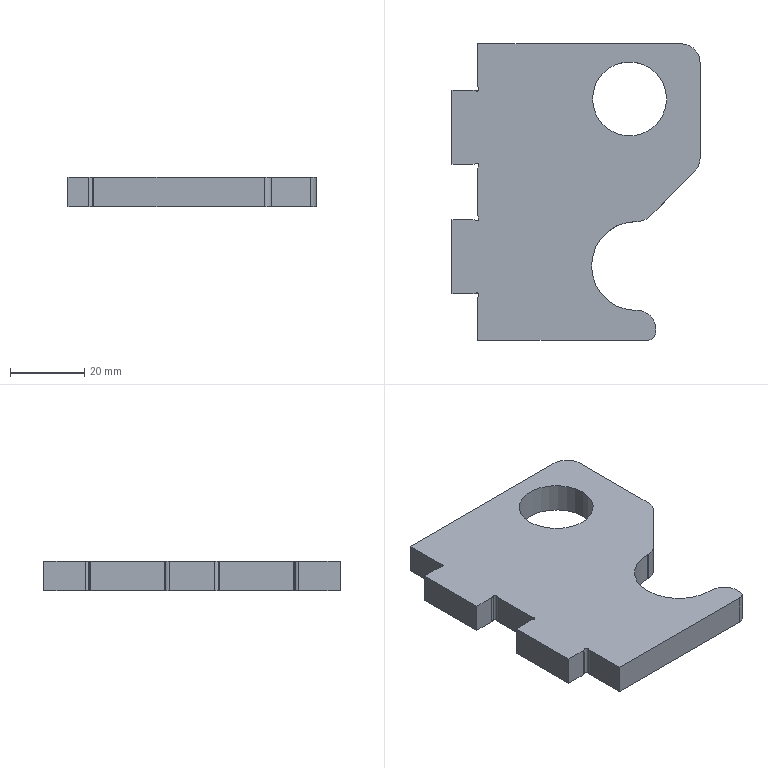Part | SolidWorks | features Fillet 2, Chamfer 1, FlatPattern 1, ICE 1, SMBaseFlange 1, SheetMetal 1 | 1 solid | 43 faces | box 67 x 80 x 8 mm | volume 31215 mm3 | cylinder 25 | plane 18 | commonest cylinder face diameters 4 x9 1 x8 10 x4 20 x2 24 x2
STEP:
#1=CARTESIAN_POINT('',(-1503.95,-7.25,0.));
#2=VERTEX_POINT('',#1);
#3=CARTESIAN_POINT('',(-1504.,-7.032,0.));
#4=VERTEX_POINT('',#3);
#5=CARTESIAN_POINT('',(-1504.45,-7.25,0.));
#6=DIRECTION('',(0.,0.,1.));
#7=DIRECTION('',(1.,0.,0.));
#8=AXIS2_PLACEMENT_3D('',#5,#6,#7);
#9=CIRCLE('',#8,0.5);
#10=EDGE_CURVE('',#2,#4,#9,.T.);
#11=ORIENTED_EDGE('',*,*,#10,.F.);
#12=CARTESIAN_POINT('',(-1503.95,-7.25,8.));
#13=VERTEX_POINT('',#12);
#14=CARTESIAN_POINT('',(-1503.95,-7.25,0.));
#15=DIRECTION('',(0.,0.,1.));
#16=VECTOR('',#15,1000.);
#17=LINE('',#14,#16);
#18=EDGE_CURVE('',#2,#13,#17,.T.);
#19=ORIENTED_EDGE('',*,*,#18,.T.);
#20=CARTESIAN_POINT('',(-1504.,-7.032,8.));
#21=VERTEX_POINT('',#20);
#22=CARTESIAN_POINT('',(-1504.45,-7.25,8.));
#23=DIRECTION('',(0.,0.,1.));
#24=DIRECTION('',(1.,0.,0.));
#25=AXIS2_PLACEMENT_3D('',#22,#23,#24);
#26=CIRCLE('',#25,0.5);
#27=EDGE_CURVE('',#13,#21,#26,.T.);
#28=ORIENTED_EDGE('',*,*,#27,.T.);
#29=CARTESIAN_POINT('',(-1504.,-7.032,0.));
#30=DIRECTION('',(0.,0.,-1.));
#31=VECTOR('',#30,1000.);
#32=LINE('',#29,#31);
#33=EDGE_CURVE('',#21,#4,#32,.T.);
#34=ORIENTED_EDGE('',*,*,#33,.T.);
#35=EDGE_LOOP('',(#11,#19,#28,#34));
#36=FACE_OUTER_BOUND('',#35,.T.);
#37=CARTESIAN_POINT('',(-1504.45,-7.25,0.));
#38=DIRECTION('',(0.,0.,1.));
#39=DIRECTION('',(1.,0.,0.));
#40=AXIS2_PLACEMENT_3D('',#37,#38,#39);
#41=CYLINDRICAL_SURFACE('',#40,0.5);
#42=ADVANCED_FACE('',(#36),#41,.F.);
#43=CARTESIAN_POINT('',(-1503.95,-27.75,0.));
#44=VERTEX_POINT('',#43);
#45=CARTESIAN_POINT('',(-1504.668,-27.3,0.));
#46=VERTEX_POINT('',#45);
#47=CARTESIAN_POINT('',(-1504.45,-27.75,0.));
#48=DIRECTION('',(0.,0.,1.));
#49=DIRECTION('',(1.,0.,0.));
#50=AXIS2_PLACEMENT_3D('',#47,#48,#49);
#51=CIRCLE('',#50,0.5);
#52=EDGE_CURVE('',#44,#46,#51,.T.);
#53=ORIENTED_EDGE('',*,*,#52,.F.);
#54=CARTESIAN_POINT('',(-1503.95,-27.75,8.));
#55=VERTEX_POINT('',#54);
#56=CARTESIAN_POINT('',(-1503.95,-27.75,0.));
#57=DIRECTION('',(0.,0.,1.));
#58=VECTOR('',#57,1000.);
#59=LINE('',#56,#58);
#60=EDGE_CURVE('',#44,#55,#59,.T.);
#61=ORIENTED_EDGE('',*,*,#60,.T.);
#62=CARTESIAN_POINT('',(-1504.668,-27.3,8.));
#63=VERTEX_POINT('',#62);
#64=CARTESIAN_POINT('',(-1504.45,-27.75,8.));
#65=DIRECTION('',(0.,0.,1.));
#66=DIRECTION('',(1.,0.,0.));
#67=AXIS2_PLACEMENT_3D('',#64,#65,#66);
#68=CIRCLE('',#67,0.5);
#69=EDGE_CURVE('',#55,#63,#68,.T.);
#70=ORIENTED_EDGE('',*,*,#69,.T.);
#71=CARTESIAN_POINT('',(-1504.668,-27.3,0.));
#72=DIRECTION('',(0.,0.,-1.));
#73=VECTOR('',#72,1000.);
#74=LINE('',#71,#73);
#75=EDGE_CURVE('',#63,#46,#74,.T.);
#76=ORIENTED_EDGE('',*,*,#75,.T.);
#77=EDGE_LOOP('',(#53,#61,#70,#76));
#78=FACE_OUTER_BOUND('',#77,.T.);
#79=CARTESIAN_POINT('',(-1504.45,-27.75,0.));
#80=DIRECTION('',(0.,0.,1.));
#81=DIRECTION('',(1.,0.,0.));
#82=AXIS2_PLACEMENT_3D('',#79,#80,#81);
#83=CYLINDRICAL_SURFACE('',#82,0.5);
#84=ADVANCED_FACE('',(#78),#83,.F.);
#85=CARTESIAN_POINT('',(-1503.95,-42.25,0.));
#86=VERTEX_POINT('',#85);
#87=CARTESIAN_POINT('',(-1504.,-42.032,0.));
#88=VERTEX_POINT('',#87);
#89=CARTESIAN_POINT('',(-1504.45,-42.25,0.));
#90=DIRECTION('',(0.,0.,1.));
#91=DIRECTION('',(1.,0.,0.));
#92=AXIS2_PLACEMENT_3D('',#89,#90,#91);
#93=CIRCLE('',#92,0.5);
#94=EDGE_CURVE('',#86,#88,#93,.T.);
#95=ORIENTED_EDGE('',*,*,#94,.F.);
#96=CARTESIAN_POINT('',(-1503.95,-42.25,8.));
#97=VERTEX_POINT('',#96);
#98=CARTESIAN_POINT('',(-1503.95,-42.25,0.));
#99=DIRECTION('',(0.,0.,1.));
#100=VECTOR('',#99,1000.);
#101=LINE('',#98,#100);
#102=EDGE_CURVE('',#86,#97,#101,.T.);
#103=ORIENTED_EDGE('',*,*,#102,.T.);
#104=CARTESIAN_POINT('',(-1504.,-42.032,8.));
#105=VERTEX_POINT('',#104);
#106=CARTESIAN_POINT('',(-1504.45,-42.25,8.));
#107=DIRECTION('',(0.,0.,1.));
#108=DIRECTION('',(1.,0.,0.));
#109=AXIS2_PLACEMENT_3D('',#106,#107,#108);
#110=CIRCLE('',#109,0.5);
#111=EDGE_CURVE('',#97,#105,#110,.T.);
#112=ORIENTED_EDGE('',*,*,#111,.T.);
#113=CARTESIAN_POINT('',(-1504.,-42.032,0.));
#114=DIRECTION('',(0.,0.,-1.));
#115=VECTOR('',#114,1000.);
#116=LINE('',#113,#115);
#117=EDGE_CURVE('',#105,#88,#116,.T.);
#118=ORIENTED_EDGE('',*,*,#117,.T.);
#119=EDGE_LOOP('',(#95,#103,#112,#118));
#120=FACE_OUTER_BOUND('',#119,.T.);
#121=CARTESIAN_POINT('',(-1504.45,-42.25,0.));
#122=DIRECTION('',(0.,0.,1.));
#123=DIRECTION('',(1.,0.,0.));
#124=AXIS2_PLACEMENT_3D('',#121,#122,#123);
#125=CYLINDRICAL_SURFACE('',#124,0.5);
#126=ADVANCED_FACE('',(#120),#125,.F.);
#127=CARTESIAN_POINT('',(-1503.95,-62.75,0.));
#128=VERTEX_POINT('',#127);
#129=CARTESIAN_POINT('',(-1504.668,-62.3,0.));
#130=VERTEX_POINT('',#129);
#131=CARTESIAN_POINT('',(-1504.45,-62.75,0.));
#132=DIRECTION('',(0.,0.,1.));
#133=DIRECTION('',(1.,0.,0.));
#134=AXIS2_PLACEMENT_3D('',#131,#132,#133);
#135=CIRCLE('',#134,0.5);
#136=EDGE_CURVE('',#128,#130,#135,.T.);
#137=ORIENTED_EDGE('',*,*,#136,.F.);
#138=CARTESIAN_POINT('',(-1503.95,-62.75,8.));
#139=VERTEX_POINT('',#138);
#140=CARTESIAN_POINT('',(-1503.95,-62.75,0.));
#141=DIRECTION('',(0.,0.,1.));
#142=VECTOR('',#141,1000.);
#143=LINE('',#140,#142);
#144=EDGE_CURVE('',#128,#139,#143,.T.);
#145=ORIENTED_EDGE('',*,*,#144,.T.);
#146=CARTESIAN_POINT('',(-1504.668,-62.3,8.));
#147=VERTEX_POINT('',#146);
#148=CARTESIAN_POINT('',(-1504.45,-62.75,8.));
#149=DIRECTION('',(0.,0.,1.));
#150=DIRECTION('',(1.,0.,0.));
#151=AXIS2_PLACEMENT_3D('',#148,#149,#150);
#152=CIRCLE('',#151,0.5);
#153=EDGE_CURVE('',#139,#147,#152,.T.);
#154=ORIENTED_EDGE('',*,*,#153,.T.);
#155=CARTESIAN_POINT('',(-1504.668,-62.3,0.));
#156=DIRECTION('',(0.,0.,-1.));
#157=VECTOR('',#156,1000.);
#158=LINE('',#155,#157);
#159=EDGE_CURVE('',#147,#130,#158,.T.);
#160=ORIENTED_EDGE('',*,*,#159,.T.);
#161=EDGE_LOOP('',(#137,#145,#154,#160));
#162=FACE_OUTER_BOUND('',#161,.T.);
#163=CARTESIAN_POINT('',(-1504.45,-62.75,0.));
#164=DIRECTION('',(0.,0.,1.));
#165=DIRECTION('',(1.,0.,0.));
#166=AXIS2_PLACEMENT_3D('',#163,#164,#165);
#167=CYLINDRICAL_SURFACE('',#166,0.5);
#168=ADVANCED_FACE('',(#162),#167,.F.);
#169=CARTESIAN_POINT('',(-1473.236,-9.864,8.));
#170=VERTEX_POINT('',#169);
#171=CARTESIAN_POINT('',(-1453.236,-9.864,8.));
#172=VERTEX_POINT('',#171);
#173=CARTESIAN_POINT('',(-1463.236,-9.864,8.));
#174=DIRECTION('',(0.,0.,1.));
#175=DIRECTION('',(1.,0.,0.));
#176=AXIS2_PLACEMENT_3D('',#173,#174,#175);
#177=CIRCLE('',#176,10.);
#178=EDGE_CURVE('',#170,#172,#177,.T.);
#179=ORIENTED_EDGE('',*,*,#178,.T.);
#180=CARTESIAN_POINT('',(-1453.236,-9.864,0.));
#181=VERTEX_POINT('',#180);
#182=CARTESIAN_POINT('',(-1453.236,-9.864,8.));
#183=DIRECTION('',(0.,0.,-1.));
#184=VECTOR('',#183,1000.);
#185=LINE('',#182,#184);
#186=EDGE_CURVE('',#172,#181,#185,.T.);
#187=ORIENTED_EDGE('',*,*,#186,.T.);
#188=CARTESIAN_POINT('',(-1473.236,-9.864,0.));
#189=VERTEX_POINT('',#188);
#190=CARTESIAN_POINT('',(-1463.236,-9.864,0.));
#191=DIRECTION('',(0.,0.,1.));
#192=DIRECTION('',(1.,0.,0.));
#193=AXIS2_PLACEMENT_3D('',#190,#191,#192);
#194=CIRCLE('',#193,10.);
#195=EDGE_CURVE('',#189,#181,#194,.T.);
#196=ORIENTED_EDGE('',*,*,#195,.F.);
#197=CARTESIAN_POINT('',(-1473.236,-9.864,8.));
#198=DIRECTION('',(0.,0.,-1.));
#199=VECTOR('',#198,1000.);
#200=LINE('',#197,#199);
#201=EDGE_CURVE('',#170,#189,#200,.T.);
#202=ORIENTED_EDGE('',*,*,#201,.F.);
#203=EDGE_LOOP('',(#179,#187,#196,#202));
#204=FACE_OUTER_BOUND('',#203,.T.);
#205=CARTESIAN_POINT('',(-1463.236,-9.864,8.));
#206=DIRECTION('',(0.,0.,-1.));
#207=DIRECTION('',(-1.,0.,0.));
#208=AXIS2_PLACEMENT_3D('',#205,#206,#207);
#209=CYLINDRICAL_SURFACE('',#208,10.);
#210=ADVANCED_FACE('',(#204),#209,.F.);
#211=CARTESIAN_POINT('',(-1473.5,-55.,8.));
#212=VERTEX_POINT('',#211);
#213=CARTESIAN_POINT('',(-1461.5,-43.,8.));
#214=VERTEX_POINT('',#213);
#215=CARTESIAN_POINT('',(-1461.5,-55.,8.));
#216=DIRECTION('',(0.,0.,-1.));
#217=DIRECTION('',(1.,0.,0.));
#218=AXIS2_PLACEMENT_3D('',#215,#216,#217);
#219=CIRCLE('',#218,12.);
#220=EDGE_CURVE('',#212,#214,#219,.T.);
#221=ORIENTED_EDGE('',*,*,#220,.F.);
#222=CARTESIAN_POINT('',(-1473.5,-55.,0.));
#223=VERTEX_POINT('',#222);
#224=CARTESIAN_POINT('',(-1473.5,-55.,8.));
#225=DIRECTION('',(0.,0.,-1.));
#226=VECTOR('',#225,1000.);
#227=LINE('',#224,#226);
#228=EDGE_CURVE('',#212,#223,#227,.T.);
#229=ORIENTED_EDGE('',*,*,#228,.T.);
#230=CARTESIAN_POINT('',(-1461.5,-43.,0.));
#231=VERTEX_POINT('',#230);
#232=CARTESIAN_POINT('',(-1461.5,-55.,0.));
#233=DIRECTION('',(0.,0.,-1.));
#234=DIRECTION('',(1.,0.,0.));
#235=AXIS2_PLACEMENT_3D('',#232,#233,#234);
#236=CIRCLE('',#235,12.);
#237=EDGE_CURVE('',#223,#231,#236,.T.);
#238=ORIENTED_EDGE('',*,*,#237,.T.);
#239=CARTESIAN_POINT('',(-1461.5,-43.,8.));
#240=DIRECTION('',(0.,0.,-1.));
#241=VECTOR('',#240,1000.);
#242=LINE('',#239,#241);
#243=EDGE_CURVE('',#214,#231,#242,.T.);
#244=ORIENTED_EDGE('',*,*,#243,.F.);
#245=EDGE_LOOP('',(#221,#229,#238,#244));
#246=FACE_OUTER_BOUND('',#245,.T.);
#247=CARTESIAN_POINT('',(-1461.5,-55.,8.));
#248=DIRECTION('',(0.,0.,-1.));
#249=DIRECTION('',(-1.,0.,0.));
#250=AXIS2_PLACEMENT_3D('',#247,#248,#249);
#251=CYLINDRICAL_SURFACE('',#250,12.);
#252=ADVANCED_FACE('',(#246),#251,.F.);
#253=ORIENTED_EDGE('',*,*,#178,.F.);
#254=CARTESIAN_POINT('',(-1463.236,-9.864,8.));
#255=DIRECTION('',(0.,0.,1.));
#256=DIRECTION('',(1.,0.,0.));
#257=AXIS2_PLACEMENT_3D('',#254,#255,#256);
#258=CIRCLE('',#257,10.);
#259=EDGE_CURVE('',#172,#170,#258,.T.);
#260=ORIENTED_EDGE('',*,*,#259,.F.);
#261=EDGE_LOOP('',(#253,#260));
#262=FACE_BOUND('',#261,.T.);
#263=CARTESIAN_POINT('',(-1444.2,-25.929,8.));
#264=VERTEX_POINT('',#263);
#265=CARTESIAN_POINT('',(-1444.2,0.,8.));
#266=VERTEX_POINT('',#265);
#267=CARTESIAN_POINT('',(-1444.2,5.,8.));
#268=DIRECTION('',(0.,1.,0.));
#269=VECTOR('',#268,1000.);
#270=LINE('',#267,#269);
#271=EDGE_CURVE('',#264,#266,#270,.T.);
#272=ORIENTED_EDGE('',*,*,#271,.T.);
#273=CARTESIAN_POINT('',(-1449.2,5.,8.));
#274=VERTEX_POINT('',#273);
#275=CARTESIAN_POINT('',(-1449.2,0.,8.));
#276=DIRECTION('',(0.,0.,1.));
#277=DIRECTION('',(1.,0.,0.));
#278=AXIS2_PLACEMENT_3D('',#275,#276,#277);
#279=CIRCLE('',#278,5.);
#280=EDGE_CURVE('',#266,#274,#279,.T.);
#281=ORIENTED_EDGE('',*,*,#280,.T.);
#282=CARTESIAN_POINT('',(-1504.2,5.,8.));
#283=VERTEX_POINT('',#282);
#284=CARTESIAN_POINT('',(-1504.2,5.,8.));
#285=DIRECTION('',(-1.,0.,0.));
#286=VECTOR('',#285,1000.);
#287=LINE('',#284,#286);
#288=EDGE_CURVE('',#274,#283,#287,.T.);
#289=ORIENTED_EDGE('',*,*,#288,.T.);
#290=CARTESIAN_POINT('',(-1504.2,-6.16,8.));
#291=VERTEX_POINT('',#290);
#292=CARTESIAN_POINT('',(-1504.2,-7.5,8.));
#293=DIRECTION('',(0.,-1.,0.));
#294=VECTOR('',#293,1000.);
#295=LINE('',#292,#294);
#296=EDGE_CURVE('',#283,#291,#295,.T.);
#297=ORIENTED_EDGE('',*,*,#296,.T.);
#298=CARTESIAN_POINT('',(-1502.2,-6.16,8.));
#299=DIRECTION('',(0.,0.,1.));
#300=DIRECTION('',(1.,0.,0.));
#301=AXIS2_PLACEMENT_3D('',#298,#299,#300);
#302=CIRCLE('',#301,2.);
#303=EDGE_CURVE('',#291,#21,#302,.T.);
#304=ORIENTED_EDGE('',*,*,#303,.T.);
#305=ORIENTED_EDGE('',*,*,#27,.F.);
#306=CARTESIAN_POINT('',(-1504.668,-7.7,8.));
#307=VERTEX_POINT('',#306);
#308=CARTESIAN_POINT('',(-1504.45,-7.25,8.));
#309=DIRECTION('',(0.,0.,1.));
#310=DIRECTION('',(1.,0.,0.));
#311=AXIS2_PLACEMENT_3D('',#308,#309,#310);
#312=CIRCLE('',#311,0.5);
#313=EDGE_CURVE('',#307,#13,#312,.T.);
#314=ORIENTED_EDGE('',*,*,#313,.F.);
#315=CARTESIAN_POINT('',(-1505.54,-7.5,8.));
#316=VERTEX_POINT('',#315);
#317=CARTESIAN_POINT('',(-1505.54,-9.5,8.));
#318=DIRECTION('',(0.,0.,1.));
#319=DIRECTION('',(1.,0.,0.));
#320=AXIS2_PLACEMENT_3D('',#317,#318,#319);
#321=CIRCLE('',#320,2.);
#322=EDGE_CURVE('',#307,#316,#321,.T.);
#323=ORIENTED_EDGE('',*,*,#322,.T.);
#324=CARTESIAN_POINT('',(-1511.2,-7.5,8.));
#325=VERTEX_POINT('',#324);
#326=CARTESIAN_POINT('',(-1504.2,-7.5,8.));
#327=DIRECTION('',(-1.,0.,0.));
#328=VECTOR('',#327,1000.);
#329=LINE('',#326,#328);
#330=EDGE_CURVE('',#316,#325,#329,.T.);
#331=ORIENTED_EDGE('',*,*,#330,.T.);
#332=CARTESIAN_POINT('',(-1511.2,-27.5,8.));
#333=VERTEX_POINT('',#332);
#334=CARTESIAN_POINT('',(-1511.2,-7.5,8.));
#335=DIRECTION('',(0.,-1.,0.));
#336=VECTOR('',#335,1000.);
#337=LINE('',#334,#336);
#338=EDGE_CURVE('',#325,#333,#337,.T.);
#339=ORIENTED_EDGE('',*,*,#338,.T.);
#340=CARTESIAN_POINT('',(-1505.54,-27.5,8.));
#341=VERTEX_POINT('',#340);
#342=CARTESIAN_POINT('',(-1511.2,-27.5,8.));
#343=DIRECTION('',(1.,0.,0.));
#344=VECTOR('',#343,1000.);
#345=LINE('',#342,#344);
#346=EDGE_CURVE('',#333,#341,#345,.T.);
#347=ORIENTED_EDGE('',*,*,#346,.T.);
#348=CARTESIAN_POINT('',(-1505.54,-25.5,8.));
#349=DIRECTION('',(0.,0.,1.));
#350=DIRECTION('',(1.,0.,0.));
#351=AXIS2_PLACEMENT_3D('',#348,#349,#350);
#352=CIRCLE('',#351,2.);
#353=EDGE_CURVE('',#341,#63,#352,.T.);
#354=ORIENTED_EDGE('',*,*,#353,.T.);
#355=ORIENTED_EDGE('',*,*,#69,.F.);
#356=CARTESIAN_POINT('',(-1504.,-27.968,8.));
#357=VERTEX_POINT('',#356);
#358=CARTESIAN_POINT('',(-1504.45,-27.75,8.));
#359=DIRECTION('',(0.,0.,1.));
#360=DIRECTION('',(1.,0.,0.));
#361=AXIS2_PLACEMENT_3D('',#358,#359,#360);
#362=CIRCLE('',#361,0.5);
#363=EDGE_CURVE('',#357,#55,#362,.T.);
#364=ORIENTED_EDGE('',*,*,#363,.F.);
#365=CARTESIAN_POINT('',(-1504.2,-28.84,8.));
#366=VERTEX_POINT('',#365);
#367=CARTESIAN_POINT('',(-1502.2,-28.84,8.));
#368=DIRECTION('',(0.,0.,1.));
#369=DIRECTION('',(1.,0.,0.));
#370=AXIS2_PLACEMENT_3D('',#367,#368,#369);
#371=CIRCLE('',#370,2.);
#372=EDGE_CURVE('',#357,#366,#371,.T.);
#373=ORIENTED_EDGE('',*,*,#372,.T.);
#374=CARTESIAN_POINT('',(-1504.2,-41.16,8.));
#375=VERTEX_POINT('',#374);
#376=CARTESIAN_POINT('',(-1504.2,-42.5,8.));
#377=DIRECTION('',(0.,-1.,0.));
#378=VECTOR('',#377,1000.);
#379=LINE('',#376,#378);
#380=EDGE_CURVE('',#366,#375,#379,.T.);
#381=ORIENTED_EDGE('',*,*,#380,.T.);
#382=CARTESIAN_POINT('',(-1502.2,-41.16,8.));
#383=DIRECTION('',(0.,0.,1.));
#384=DIRECTION('',(1.,0.,0.));
#385=AXIS2_PLACEMENT_3D('',#382,#383,#384);
#386=CIRCLE('',#385,2.);
#387=EDGE_CURVE('',#375,#105,#386,.T.);
#388=ORIENTED_EDGE('',*,*,#387,.T.);
#389=ORIENTED_EDGE('',*,*,#111,.F.);
#390=CARTESIAN_POINT('',(-1504.668,-42.7,8.));
#391=VERTEX_POINT('',#390);
#392=CARTESIAN_POINT('',(-1504.45,-42.25,8.));
#393=DIRECTION('',(0.,0.,1.));
#394=DIRECTION('',(1.,0.,0.));
#395=AXIS2_PLACEMENT_3D('',#392,#393,#394);
#396=CIRCLE('',#395,0.5);
#397=EDGE_CURVE('',#391,#97,#396,.T.);
#398=ORIENTED_EDGE('',*,*,#397,.F.);
#399=CARTESIAN_POINT('',(-1505.54,-42.5,8.));
#400=VERTEX_POINT('',#399);
#401=CARTESIAN_POINT('',(-1505.54,-44.5,8.));
#402=DIRECTION('',(0.,0.,1.));
#403=DIRECTION('',(1.,0.,0.));
#404=AXIS2_PLACEMENT_3D('',#401,#402,#403);
#405=CIRCLE('',#404,2.);
#406=EDGE_CURVE('',#391,#400,#405,.T.);
#407=ORIENTED_EDGE('',*,*,#406,.T.);
#408=CARTESIAN_POINT('',(-1511.2,-42.5,8.));
#409=VERTEX_POINT('',#408);
#410=CARTESIAN_POINT('',(-1511.2,-42.5,8.));
#411=DIRECTION('',(-1.,0.,0.));
#412=VECTOR('',#411,1000.);
#413=LINE('',#410,#412);
#414=EDGE_CURVE('',#400,#409,#413,.T.);
#415=ORIENTED_EDGE('',*,*,#414,.T.);
#416=CARTESIAN_POINT('',(-1511.2,-62.5,8.));
#417=VERTEX_POINT('',#416);
#418=CARTESIAN_POINT('',(-1511.2,-62.5,8.));
#419=DIRECTION('',(0.,-1.,0.));
#420=VECTOR('',#419,1000.);
#421=LINE('',#418,#420);
#422=EDGE_CURVE('',#409,#417,#421,.T.);
#423=ORIENTED_EDGE('',*,*,#422,.T.);
#424=CARTESIAN_POINT('',(-1505.54,-62.5,8.));
#425=VERTEX_POINT('',#424);
#426=CARTESIAN_POINT('',(-1504.2,-62.5,8.));
#427=DIRECTION('',(1.,0.,0.));
#428=VECTOR('',#427,1000.);
#429=LINE('',#426,#428);
#430=EDGE_CURVE('',#417,#425,#429,.T.);
#431=ORIENTED_EDGE('',*,*,#430,.T.);
#432=CARTESIAN_POINT('',(-1505.54,-60.5,8.));
#433=DIRECTION('',(0.,0.,1.));
#434=DIRECTION('',(1.,0.,0.));
#435=AXIS2_PLACEMENT_3D('',#432,#433,#434);
#436=CIRCLE('',#435,2.);
#437=EDGE_CURVE('',#425,#147,#436,.T.);
#438=ORIENTED_EDGE('',*,*,#437,.T.);
#439=ORIENTED_EDGE('',*,*,#153,.F.);
#440=CARTESIAN_POINT('',(-1504.,-62.968,8.));
#441=VERTEX_POINT('',#440);
#442=CARTESIAN_POINT('',(-1504.45,-62.75,8.));
#443=DIRECTION('',(0.,0.,1.));
#444=DIRECTION('',(1.,0.,0.));
#445=AXIS2_PLACEMENT_3D('',#442,#443,#444);
#446=CIRCLE('',#445,0.5);
#447=EDGE_CURVE('',#441,#139,#446,.T.);
#448=ORIENTED_EDGE('',*,*,#447,.F.);
#449=CARTESIAN_POINT('',(-1504.2,-63.84,8.));
#450=VERTEX_POINT('',#449);
#451=CARTESIAN_POINT('',(-1502.2,-63.84,8.));
#452=DIRECTION('',(0.,0.,1.));
#453=DIRECTION('',(1.,0.,0.));
#454=AXIS2_PLACEMENT_3D('',#451,#452,#453);
#455=CIRCLE('',#454,2.);
#456=EDGE_CURVE('',#441,#450,#455,.T.);
#457=ORIENTED_EDGE('',*,*,#456,.T.);
#458=CARTESIAN_POINT('',(-1504.2,-75.,8.));
#459=VERTEX_POINT('',#458);
#460=CARTESIAN_POINT('',(-1504.2,-75.,8.));
#461=DIRECTION('',(0.,-1.,0.));
#462=VECTOR('',#461,1000.);
#463=LINE('',#460,#462);
#464=EDGE_CURVE('',#450,#459,#463,.T.);
#465=ORIENTED_EDGE('',*,*,#464,.T.);
#466=CARTESIAN_POINT('',(-1458.2,-75.,8.));
#467=VERTEX_POINT('',#466);
#468=CARTESIAN_POINT('',(-1456.2,-75.,8.));
#469=DIRECTION('',(1.,0.,0.));
#470=VECTOR('',#469,1000.);
#471=LINE('',#468,#470);
#472=EDGE_CURVE('',#459,#467,#471,.T.);
#473=ORIENTED_EDGE('',*,*,#472,.T.);
#474=CARTESIAN_POINT('',(-1456.2,-73.,8.));
#475=VERTEX_POINT('',#474);
#476=CARTESIAN_POINT('',(-1458.2,-73.,8.));
#477=DIRECTION('',(0.,0.,1.));
#478=DIRECTION('',(1.,0.,0.));
#479=AXIS2_PLACEMENT_3D('',#476,#477,#478);
#480=CIRCLE('',#479,2.);
#481=EDGE_CURVE('',#467,#475,#480,.T.);
#482=ORIENTED_EDGE('',*,*,#481,.T.);
#483=CARTESIAN_POINT('',(-1456.2,-72.,8.));
#484=VERTEX_POINT('',#483);
#485=CARTESIAN_POINT('',(-1456.2,-67.,8.));
#486=DIRECTION('',(0.,1.,0.));
#487=VECTOR('',#486,1000.);
#488=LINE('',#485,#487);
#489=EDGE_CURVE('',#475,#484,#488,.T.);
#490=ORIENTED_EDGE('',*,*,#489,.T.);
#491=CARTESIAN_POINT('',(-1461.2,-67.,8.));
#492=VERTEX_POINT('',#491);
#493=CARTESIAN_POINT('',(-1461.2,-72.,8.));
#494=DIRECTION('',(0.,0.,1.));
#495=DIRECTION('',(1.,0.,0.));
#496=AXIS2_PLACEMENT_3D('',#493,#494,#495);
#497=CIRCLE('',#496,5.);
#498=EDGE_CURVE('',#484,#492,#497,.T.);
#499=ORIENTED_EDGE('',*,*,#498,.T.);
#500=CARTESIAN_POINT('',(-1461.5,-67.,8.));
#501=VERTEX_POINT('',#500);
#502=CARTESIAN_POINT('',(-1461.5,-67.,8.));
#503=DIRECTION('',(-1.,0.,0.));
#504=VECTOR('',#503,1000.);
#505=LINE('',#502,#504);
#506=EDGE_CURVE('',#492,#501,#505,.T.);
#507=ORIENTED_EDGE('',*,*,#506,.T.);
#508=CARTESIAN_POINT('',(-1461.5,-55.,8.));
#509=DIRECTION('',(0.,0.,-1.));
#510=DIRECTION('',(1.,0.,0.));
#511=AXIS2_PLACEMENT_3D('',#508,#509,#510);
#512=CIRCLE('',#511,12.);
#513=EDGE_CURVE('',#501,#212,#512,.T.);
#514=ORIENTED_EDGE('',*,*,#513,.T.);
#515=ORIENTED_EDGE('',*,*,#220,.T.);
#516=CARTESIAN_POINT('',(-1461.271,-43.,8.));
#517=VERTEX_POINT('',#516);
#518=CARTESIAN_POINT('',(-1461.5,-43.,8.));
#519=DIRECTION('',(1.,0.,0.));
#520=VECTOR('',#519,1000.);
#521=LINE('',#518,#520);
#522=EDGE_CURVE('',#214,#517,#521,.T.);
#523=ORIENTED_EDGE('',*,*,#522,.T.);
#524=CARTESIAN_POINT('',(-1457.736,-41.536,8.));
#525=VERTEX_POINT('',#524);
#526=CARTESIAN_POINT('',(-1461.271,-38.,8.));
#527=DIRECTION('',(0.,0.,1.));
#528=DIRECTION('',(1.,0.,0.));
#529=AXIS2_PLACEMENT_3D('',#526,#527,#528);
#530=CIRCLE('',#529,5.);
#531=EDGE_CURVE('',#517,#525,#530,.T.);
#532=ORIENTED_EDGE('',*,*,#531,.T.);
#533=CARTESIAN_POINT('',(-1445.664,-29.464,8.));
#534=VERTEX_POINT('',#533);
#535=CARTESIAN_POINT('',(-1466.35,-50.15,8.));
#536=DIRECTION('',(0.7071,0.7071,0.));
#537=VECTOR('',#536,1000.);
#538=LINE('',#535,#537);
#539=EDGE_CURVE('',#525,#534,#538,.T.);
#540=ORIENTED_EDGE('',*,*,#539,.T.);
#541=CARTESIAN_POINT('',(-1449.2,-25.929,8.));
#542=DIRECTION('',(0.,0.,1.));
#543=DIRECTION('',(1.,0.,0.));
#544=AXIS2_PLACEMENT_3D('',#541,#542,#543);
#545=CIRCLE('',#544,5.);
#546=EDGE_CURVE('',#534,#264,#545,.T.);
#547=ORIENTED_EDGE('',*,*,#546,.T.);
#548=EDGE_LOOP('',(#272,#281,#289,#297,#304,#305,#314,#323,#331,#339,#347,#354,#355,#364,#373,#381,#388,#389,#398,#407,#415,#423,#431,#438,#439,#448,#457,#465,#473,#482,#490,#499,#507,#514,#515,#523,#532,#540,#547));
#549=FACE_OUTER_BOUND('',#548,.T.);
#550=CARTESIAN_POINT('',(-1461.5,-55.,8.));
#551=DIRECTION('',(0.,0.,1.));
#552=DIRECTION('',(1.,0.,0.));
#553=AXIS2_PLACEMENT_3D('',#550,#551,#552);
#554=PLANE('',#553);
#555=ADVANCED_FACE('',(#262,#549),#554,.T.);
#556=ORIENTED_EDGE('',*,*,#195,.T.);
#557=CARTESIAN_POINT('',(-1463.236,-9.864,0.));
#558=DIRECTION('',(0.,0.,1.));
#559=DIRECTION('',(1.,0.,0.));
#560=AXIS2_PLACEMENT_3D('',#557,#558,#559);
#561=CIRCLE('',#560,10.);
#562=EDGE_CURVE('',#181,#189,#561,.T.);
#563=ORIENTED_EDGE('',*,*,#562,.T.);
#564=EDGE_LOOP('',(#556,#563));
#565=FACE_BOUND('',#564,.T.);
#566=CARTESIAN_POINT('',(-1449.2,5.,0.));
#567=VERTEX_POINT('',#566);
#568=CARTESIAN_POINT('',(-1504.2,5.,0.));
#569=VERTEX_POINT('',#568);
#570=CARTESIAN_POINT('',(-1504.2,5.,0.));
#571=DIRECTION('',(-1.,0.,0.));
#572=VECTOR('',#571,1000.);
#573=LINE('',#570,#572);
#574=EDGE_CURVE('',#567,#569,#573,.T.);
#575=ORIENTED_EDGE('',*,*,#574,.F.);
#576=CARTESIAN_POINT('',(-1444.2,0.,0.));
#577=VERTEX_POINT('',#576);
#578=CARTESIAN_POINT('',(-1449.2,0.,0.));
#579=DIRECTION('',(0.,0.,-1.));
#580=DIRECTION('',(1.,0.,0.));
#581=AXIS2_PLACEMENT_3D('',#578,#579,#580);
#582=CIRCLE('',#581,5.);
#583=EDGE_CURVE('',#567,#577,#582,.T.);
#584=ORIENTED_EDGE('',*,*,#583,.T.);
#585=CARTESIAN_POINT('',(-1444.2,-25.929,0.));
#586=VERTEX_POINT('',#585);
#587=CARTESIAN_POINT('',(-1444.2,5.,0.));
#588=DIRECTION('',(0.,1.,0.));
#589=VECTOR('',#588,1000.);
#590=LINE('',#587,#589);
#591=EDGE_CURVE('',#586,#577,#590,.T.);
#592=ORIENTED_EDGE('',*,*,#591,.F.);
#593=CARTESIAN_POINT('',(-1445.664,-29.464,0.));
#594=VERTEX_POINT('',#593);
#595=CARTESIAN_POINT('',(-1449.2,-25.929,0.));
#596=DIRECTION('',(0.,0.,-1.));
#597=DIRECTION('',(1.,0.,0.));
#598=AXIS2_PLACEMENT_3D('',#595,#596,#597);
#599=CIRCLE('',#598,5.);
#600=EDGE_CURVE('',#586,#594,#599,.T.);
#601=ORIENTED_EDGE('',*,*,#600,.T.);
#602=CARTESIAN_POINT('',(-1457.736,-41.536,0.));
#603=VERTEX_POINT('',#602);
#604=CARTESIAN_POINT('',(-1444.2,-28.,0.));
#605=DIRECTION('',(-0.7071,-0.7071,0.));
#606=VECTOR('',#605,1000.);
#607=LINE('',#604,#606);
#608=EDGE_CURVE('',#594,#603,#607,.T.);
#609=ORIENTED_EDGE('',*,*,#608,.T.);
#610=CARTESIAN_POINT('',(-1461.271,-43.,0.));
#611=VERTEX_POINT('',#610);
#612=CARTESIAN_POINT('',(-1461.271,-38.,0.));
#613=DIRECTION('',(0.,0.,-1.));
#614=DIRECTION('',(1.,0.,0.));
#615=AXIS2_PLACEMENT_3D('',#612,#613,#614);
#616=CIRCLE('',#615,5.);
#617=EDGE_CURVE('',#603,#611,#616,.T.);
#618=ORIENTED_EDGE('',*,*,#617,.T.);
#619=CARTESIAN_POINT('',(-1461.5,-43.,0.));
#620=DIRECTION('',(1.,0.,0.));
#621=VECTOR('',#620,1000.);
#622=LINE('',#619,#621);
#623=EDGE_CURVE('',#231,#611,#622,.T.);
#624=ORIENTED_EDGE('',*,*,#623,.F.);
#625=ORIENTED_EDGE('',*,*,#237,.F.);
#626=CARTESIAN_POINT('',(-1461.5,-67.,0.));
#627=VERTEX_POINT('',#626);
#628=CARTESIAN_POINT('',(-1461.5,-55.,0.));
#629=DIRECTION('',(0.,0.,-1.));
#630=DIRECTION('',(1.,0.,0.));
#631=AXIS2_PLACEMENT_3D('',#628,#629,#630);
#632=CIRCLE('',#631,12.);
#633=EDGE_CURVE('',#627,#223,#632,.T.);
#634=ORIENTED_EDGE('',*,*,#633,.F.);
#635=CARTESIAN_POINT('',(-1461.2,-67.,0.));
#636=VERTEX_POINT('',#635);
#637=CARTESIAN_POINT('',(-1461.5,-67.,0.));
#638=DIRECTION('',(-1.,0.,0.));
#639=VECTOR('',#638,1000.);
#640=LINE('',#637,#639);
#641=EDGE_CURVE('',#636,#627,#640,.T.);
#642=ORIENTED_EDGE('',*,*,#641,.F.);
#643=CARTESIAN_POINT('',(-1456.2,-72.,0.));
#644=VERTEX_POINT('',#643);
#645=CARTESIAN_POINT('',(-1461.2,-72.,0.));
#646=DIRECTION('',(0.,0.,-1.));
#647=DIRECTION('',(1.,0.,0.));
#648=AXIS2_PLACEMENT_3D('',#645,#646,#647);
#649=CIRCLE('',#648,5.);
#650=EDGE_CURVE('',#636,#644,#649,.T.);
#651=ORIENTED_EDGE('',*,*,#650,.T.);
#652=CARTESIAN_POINT('',(-1456.2,-73.,0.));
#653=VERTEX_POINT('',#652);
#654=CARTESIAN_POINT('',(-1456.2,-67.,0.));
#655=DIRECTION('',(0.,1.,0.));
#656=VECTOR('',#655,1000.);
#657=LINE('',#654,#656);
#658=EDGE_CURVE('',#653,#644,#657,.T.);
#659=ORIENTED_EDGE('',*,*,#658,.F.);
#660=CARTESIAN_POINT('',(-1458.2,-75.,0.));
#661=VERTEX_POINT('',#660);
#662=CARTESIAN_POINT('',(-1458.2,-73.,0.));
#663=DIRECTION('',(0.,0.,-1.));
#664=DIRECTION('',(1.,0.,0.));
#665=AXIS2_PLACEMENT_3D('',#662,#663,#664);
#666=CIRCLE('',#665,2.);
#667=EDGE_CURVE('',#653,#661,#666,.T.);
#668=ORIENTED_EDGE('',*,*,#667,.T.);
#669=CARTESIAN_POINT('',(-1504.2,-75.,0.));
#670=VERTEX_POINT('',#669);
#671=CARTESIAN_POINT('',(-1456.2,-75.,0.));
#672=DIRECTION('',(1.,0.,0.));
#673=VECTOR('',#672,1000.);
#674=LINE('',#671,#673);
#675=EDGE_CURVE('',#670,#661,#674,.T.);
#676=ORIENTED_EDGE('',*,*,#675,.F.);
#677=CARTESIAN_POINT('',(-1504.2,-63.84,0.));
#678=VERTEX_POINT('',#677);
#679=CARTESIAN_POINT('',(-1504.2,-75.,0.));
#680=DIRECTION('',(0.,-1.,0.));
#681=VECTOR('',#680,1000.);
#682=LINE('',#679,#681);
#683=EDGE_CURVE('',#678,#670,#682,.T.);
#684=ORIENTED_EDGE('',*,*,#683,.F.);
#685=CARTESIAN_POINT('',(-1504.,-62.968,0.));
#686=VERTEX_POINT('',#685);
#687=CARTESIAN_POINT('',(-1502.2,-63.84,0.));
#688=DIRECTION('',(0.,0.,-1.));
#689=DIRECTION('',(1.,0.,0.));
#690=AXIS2_PLACEMENT_3D('',#687,#688,#689);
#691=CIRCLE('',#690,2.);
#692=EDGE_CURVE('',#678,#686,#691,.T.);
#693=ORIENTED_EDGE('',*,*,#692,.T.);
#694=CARTESIAN_POINT('',(-1504.45,-62.75,0.));
#695=DIRECTION('',(0.,0.,1.));
#696=DIRECTION('',(1.,0.,0.));
#697=AXIS2_PLACEMENT_3D('',#694,#695,#696);
#698=CIRCLE('',#697,0.5);
#699=EDGE_CURVE('',#686,#128,#698,.T.);
#700=ORIENTED_EDGE('',*,*,#699,.T.);
#701=ORIENTED_EDGE('',*,*,#136,.T.);
#702=CARTESIAN_POINT('',(-1505.54,-62.5,0.));
#703=VERTEX_POINT('',#702);
#704=CARTESIAN_POINT('',(-1505.54,-60.5,0.));
#705=DIRECTION('',(0.,0.,-1.));
#706=DIRECTION('',(1.,0.,0.));
#707=AXIS2_PLACEMENT_3D('',#704,#705,#706);
#708=CIRCLE('',#707,2.);
#709=EDGE_CURVE('',#130,#703,#708,.T.);
#710=ORIENTED_EDGE('',*,*,#709,.T.);
#711=CARTESIAN_POINT('',(-1511.2,-62.5,0.));
#712=VERTEX_POINT('',#711);
#713=CARTESIAN_POINT('',(-1504.2,-62.5,0.));
#714=DIRECTION('',(1.,0.,0.));
#715=VECTOR('',#714,1000.);
#716=LINE('',#713,#715);
#717=EDGE_CURVE('',#712,#703,#716,.T.);
#718=ORIENTED_EDGE('',*,*,#717,.F.);
#719=CARTESIAN_POINT('',(-1511.2,-42.5,0.));
#720=VERTEX_POINT('',#719);
#721=CARTESIAN_POINT('',(-1511.2,-62.5,0.));
#722=DIRECTION('',(0.,-1.,0.));
#723=VECTOR('',#722,1000.);
#724=LINE('',#721,#723);
#725=EDGE_CURVE('',#720,#712,#724,.T.);
#726=ORIENTED_EDGE('',*,*,#725,.F.);
#727=CARTESIAN_POINT('',(-1505.54,-42.5,0.));
#728=VERTEX_POINT('',#727);
#729=CARTESIAN_POINT('',(-1511.2,-42.5,0.));
#730=DIRECTION('',(-1.,0.,0.));
#731=VECTOR('',#730,1000.);
#732=LINE('',#729,#731);
#733=EDGE_CURVE('',#728,#720,#732,.T.);
#734=ORIENTED_EDGE('',*,*,#733,.F.);
#735=CARTESIAN_POINT('',(-1504.668,-42.7,0.));
#736=VERTEX_POINT('',#735);
#737=CARTESIAN_POINT('',(-1505.54,-44.5,0.));
#738=DIRECTION('',(0.,0.,-1.));
#739=DIRECTION('',(1.,0.,0.));
#740=AXIS2_PLACEMENT_3D('',#737,#738,#739);
#741=CIRCLE('',#740,2.);
#742=EDGE_CURVE('',#728,#736,#741,.T.);
#743=ORIENTED_EDGE('',*,*,#742,.T.);
#744=CARTESIAN_POINT('',(-1504.45,-42.25,0.));
#745=DIRECTION('',(0.,0.,1.));
#746=DIRECTION('',(1.,0.,0.));
#747=AXIS2_PLACEMENT_3D('',#744,#745,#746);
#748=CIRCLE('',#747,0.5);
#749=EDGE_CURVE('',#736,#86,#748,.T.);
#750=ORIENTED_EDGE('',*,*,#749,.T.);
#751=ORIENTED_EDGE('',*,*,#94,.T.);
#752=CARTESIAN_POINT('',(-1504.2,-41.16,0.));
#753=VERTEX_POINT('',#752);
#754=CARTESIAN_POINT('',(-1502.2,-41.16,0.));
#755=DIRECTION('',(0.,0.,-1.));
#756=DIRECTION('',(1.,0.,0.));
#757=AXIS2_PLACEMENT_3D('',#754,#755,#756);
#758=CIRCLE('',#757,2.);
#759=EDGE_CURVE('',#88,#753,#758,.T.);
#760=ORIENTED_EDGE('',*,*,#759,.T.);
#761=CARTESIAN_POINT('',(-1504.2,-28.84,0.));
#762=VERTEX_POINT('',#761);
#763=CARTESIAN_POINT('',(-1504.2,-42.5,0.));
#764=DIRECTION('',(0.,-1.,0.));
#765=VECTOR('',#764,1000.);
#766=LINE('',#763,#765);
#767=EDGE_CURVE('',#762,#753,#766,.T.);
#768=ORIENTED_EDGE('',*,*,#767,.F.);
#769=CARTESIAN_POINT('',(-1504.,-27.968,0.));
#770=VERTEX_POINT('',#769);
#771=CARTESIAN_POINT('',(-1502.2,-28.84,0.));
#772=DIRECTION('',(0.,0.,-1.));
#773=DIRECTION('',(1.,0.,0.));
#774=AXIS2_PLACEMENT_3D('',#771,#772,#773);
#775=CIRCLE('',#774,2.);
#776=EDGE_CURVE('',#762,#770,#775,.T.);
#777=ORIENTED_EDGE('',*,*,#776,.T.);
#778=CARTESIAN_POINT('',(-1504.45,-27.75,0.));
#779=DIRECTION('',(0.,0.,1.));
#780=DIRECTION('',(1.,0.,0.));
#781=AXIS2_PLACEMENT_3D('',#778,#779,#780);
#782=CIRCLE('',#781,0.5);
#783=EDGE_CURVE('',#770,#44,#782,.T.);
#784=ORIENTED_EDGE('',*,*,#783,.T.);
#785=ORIENTED_EDGE('',*,*,#52,.T.);
#786=CARTESIAN_POINT('',(-1505.54,-27.5,0.));
#787=VERTEX_POINT('',#786);
#788=CARTESIAN_POINT('',(-1505.54,-25.5,0.));
#789=DIRECTION('',(0.,0.,-1.));
#790=DIRECTION('',(1.,0.,0.));
#791=AXIS2_PLACEMENT_3D('',#788,#789,#790);
#792=CIRCLE('',#791,2.);
#793=EDGE_CURVE('',#46,#787,#792,.T.);
#794=ORIENTED_EDGE('',*,*,#793,.T.);
#795=CARTESIAN_POINT('',(-1511.2,-27.5,0.));
#796=VERTEX_POINT('',#795);
#797=CARTESIAN_POINT('',(-1511.2,-27.5,0.));
#798=DIRECTION('',(1.,0.,0.));
#799=VECTOR('',#798,1000.);
#800=LINE('',#797,#799);
#801=EDGE_CURVE('',#796,#787,#800,.T.);
#802=ORIENTED_EDGE('',*,*,#801,.F.);
#803=CARTESIAN_POINT('',(-1511.2,-7.5,0.));
#804=VERTEX_POINT('',#803);
#805=CARTESIAN_POINT('',(-1511.2,-7.5,0.));
#806=DIRECTION('',(0.,-1.,0.));
#807=VECTOR('',#806,1000.);
#808=LINE('',#805,#807);
#809=EDGE_CURVE('',#804,#796,#808,.T.);
#810=ORIENTED_EDGE('',*,*,#809,.F.);
#811=CARTESIAN_POINT('',(-1505.54,-7.5,0.));
#812=VERTEX_POINT('',#811);
#813=CARTESIAN_POINT('',(-1504.2,-7.5,0.));
#814=DIRECTION('',(-1.,0.,0.));
#815=VECTOR('',#814,1000.);
#816=LINE('',#813,#815);
#817=EDGE_CURVE('',#812,#804,#816,.T.);
#818=ORIENTED_EDGE('',*,*,#817,.F.);
#819=CARTESIAN_POINT('',(-1504.668,-7.7,0.));
#820=VERTEX_POINT('',#819);
#821=CARTESIAN_POINT('',(-1505.54,-9.5,0.));
#822=DIRECTION('',(0.,0.,-1.));
#823=DIRECTION('',(1.,0.,0.));
#824=AXIS2_PLACEMENT_3D('',#821,#822,#823);
#825=CIRCLE('',#824,2.);
#826=EDGE_CURVE('',#812,#820,#825,.T.);
#827=ORIENTED_EDGE('',*,*,#826,.T.);
#828=CARTESIAN_POINT('',(-1504.45,-7.25,0.));
#829=DIRECTION('',(0.,0.,1.));
#830=DIRECTION('',(1.,0.,0.));
#831=AXIS2_PLACEMENT_3D('',#828,#829,#830);
#832=CIRCLE('',#831,0.5);
#833=EDGE_CURVE('',#820,#2,#832,.T.);
#834=ORIENTED_EDGE('',*,*,#833,.T.);
#835=ORIENTED_EDGE('',*,*,#10,.T.);
#836=CARTESIAN_POINT('',(-1504.2,-6.16,0.));
#837=VERTEX_POINT('',#836);
#838=CARTESIAN_POINT('',(-1502.2,-6.16,0.));
#839=DIRECTION('',(0.,0.,-1.));
#840=DIRECTION('',(1.,0.,0.));
#841=AXIS2_PLACEMENT_3D('',#838,#839,#840);
#842=CIRCLE('',#841,2.);
#843=EDGE_CURVE('',#4,#837,#842,.T.);
#844=ORIENTED_EDGE('',*,*,#843,.T.);
#845=CARTESIAN_POINT('',(-1504.2,-7.5,0.));
#846=DIRECTION('',(0.,-1.,0.));
#847=VECTOR('',#846,1000.);
#848=LINE('',#845,#847);
#849=EDGE_CURVE('',#569,#837,#848,.T.);
#850=ORIENTED_EDGE('',*,*,#849,.F.);
#851=EDGE_LOOP('',(#575,#584,#592,#601,#609,#618,#624,#625,#634,#642,#651,#659,#668,#676,#684,#693,#700,#701,#710,#718,#726,#734,#743,#750,#751,#760,#768,#777,#784,#785,#794,#802,#810,#818,#827,#834,#835,#844,#850));
#852=FACE_OUTER_BOUND('',#851,.T.);
#853=CARTESIAN_POINT('',(-1461.5,-55.,0.));
#854=DIRECTION('',(0.,0.,1.));
#855=DIRECTION('',(1.,0.,0.));
#856=AXIS2_PLACEMENT_3D('',#853,#854,#855);
#857=PLANE('',#856);
#858=ADVANCED_FACE('',(#565,#852),#857,.F.);
#859=ORIENTED_EDGE('',*,*,#849,.T.);
#860=CARTESIAN_POINT('',(-1504.2,-6.16,8.));
#861=DIRECTION('',(0.,0.,1.));
#862=VECTOR('',#861,1000.);
#863=LINE('',#860,#862);
#864=EDGE_CURVE('',#837,#291,#863,.T.);
#865=ORIENTED_EDGE('',*,*,#864,.T.);
#866=ORIENTED_EDGE('',*,*,#296,.F.);
#867=CARTESIAN_POINT('',(-1504.2,5.,8.));
#868=DIRECTION('',(0.,0.,-1.));
#869=VECTOR('',#868,1000.);
#870=LINE('',#867,#869);
#871=EDGE_CURVE('',#283,#569,#870,.T.);
#872=ORIENTED_EDGE('',*,*,#871,.T.);
#873=EDGE_LOOP('',(#859,#865,#866,#872));
#874=FACE_OUTER_BOUND('',#873,.T.);
#875=CARTESIAN_POINT('',(-1504.2,-7.5,8.));
#876=DIRECTION('',(1.,0.,0.));
#877=DIRECTION('',(0.,0.,-1.));
#878=AXIS2_PLACEMENT_3D('',#875,#876,#877);
#879=PLANE('',#878);
#880=ADVANCED_FACE('',(#874),#879,.F.);
#881=ORIENTED_EDGE('',*,*,#330,.F.);
#882=CARTESIAN_POINT('',(-1505.54,-7.5,0.));
#883=DIRECTION('',(0.,0.,-1.));
#884=VECTOR('',#883,1000.);
#885=LINE('',#882,#884);
#886=EDGE_CURVE('',#316,#812,#885,.T.);
#887=ORIENTED_EDGE('',*,*,#886,.T.);
#888=ORIENTED_EDGE('',*,*,#817,.T.);
#889=CARTESIAN_POINT('',(-1511.2,-7.5,8.));
#890=DIRECTION('',(0.,0.,-1.));
#891=VECTOR('',#890,1000.);
#892=LINE('',#889,#891);
#893=EDGE_CURVE('',#325,#804,#892,.T.);
#894=ORIENTED_EDGE('',*,*,#893,.F.);
#895=EDGE_LOOP('',(#881,#887,#888,#894));
#896=FACE_OUTER_BOUND('',#895,.T.);
#897=CARTESIAN_POINT('',(-1504.2,-7.5,8.));
#898=DIRECTION('',(0.,-1.,0.));
#899=DIRECTION('',(1.,0.,0.));
#900=AXIS2_PLACEMENT_3D('',#897,#898,#899);
#901=PLANE('',#900);
#902=ADVANCED_FACE('',(#896),#901,.F.);
#903=ORIENTED_EDGE('',*,*,#801,.T.);
#904=CARTESIAN_POINT('',(-1505.54,-27.5,8.));
#905=DIRECTION('',(0.,0.,1.));
#906=VECTOR('',#905,1000.);
#907=LINE('',#904,#906);
#908=EDGE_CURVE('',#787,#341,#907,.T.);
#909=ORIENTED_EDGE('',*,*,#908,.T.);
#910=ORIENTED_EDGE('',*,*,#346,.F.);
#911=CARTESIAN_POINT('',(-1511.2,-27.5,8.));
#912=DIRECTION('',(0.,0.,-1.));
#913=VECTOR('',#912,1000.);
#914=LINE('',#911,#913);
#915=EDGE_CURVE('',#333,#796,#914,.T.);
#916=ORIENTED_EDGE('',*,*,#915,.T.);
#917=EDGE_LOOP('',(#903,#909,#910,#916));
#918=FACE_OUTER_BOUND('',#917,.T.);
#919=CARTESIAN_POINT('',(-1511.2,-27.5,8.));
#920=DIRECTION('',(0.,1.,0.));
#921=DIRECTION('',(0.,0.,1.));
#922=AXIS2_PLACEMENT_3D('',#919,#920,#921);
#923=PLANE('',#922);
#924=ADVANCED_FACE('',(#918),#923,.F.);
#925=ORIENTED_EDGE('',*,*,#767,.T.);
#926=CARTESIAN_POINT('',(-1504.2,-41.16,8.));
#927=DIRECTION('',(0.,0.,1.));
#928=VECTOR('',#927,1000.);
#929=LINE('',#926,#928);
#930=EDGE_CURVE('',#753,#375,#929,.T.);
#931=ORIENTED_EDGE('',*,*,#930,.T.);
#932=ORIENTED_EDGE('',*,*,#380,.F.);
#933=CARTESIAN_POINT('',(-1504.2,-28.84,0.));
#934=DIRECTION('',(0.,0.,-1.));
#935=VECTOR('',#934,1000.);
#936=LINE('',#933,#935);
#937=EDGE_CURVE('',#366,#762,#936,.T.);
#938=ORIENTED_EDGE('',*,*,#937,.T.);
#939=EDGE_LOOP('',(#925,#931,#932,#938));
#940=FACE_OUTER_BOUND('',#939,.T.);
#941=CARTESIAN_POINT('',(-1504.2,-42.5,8.));
#942=DIRECTION('',(1.,0.,0.));
#943=DIRECTION('',(0.,0.,-1.));
#944=AXIS2_PLACEMENT_3D('',#941,#942,#943);
#945=PLANE('',#944);
#946=ADVANCED_FACE('',(#940),#945,.F.);
#947=ORIENTED_EDGE('',*,*,#414,.F.);
#948=CARTESIAN_POINT('',(-1505.54,-42.5,0.));
#949=DIRECTION('',(0.,0.,-1.));
#950=VECTOR('',#949,1000.);
#951=LINE('',#948,#950);
#952=EDGE_CURVE('',#400,#728,#951,.T.);
#953=ORIENTED_EDGE('',*,*,#952,.T.);
#954=ORIENTED_EDGE('',*,*,#733,.T.);
#955=CARTESIAN_POINT('',(-1511.2,-42.5,8.));
#956=DIRECTION('',(0.,0.,-1.));
#957=VECTOR('',#956,1000.);
#958=LINE('',#955,#957);
#959=EDGE_CURVE('',#409,#720,#958,.T.);
#960=ORIENTED_EDGE('',*,*,#959,.F.);
#961=EDGE_LOOP('',(#947,#953,#954,#960));
#962=FACE_OUTER_BOUND('',#961,.T.);
#963=CARTESIAN_POINT('',(-1511.2,-42.5,8.));
#964=DIRECTION('',(0.,-1.,0.));
#965=DIRECTION('',(0.,0.,-1.));
#966=AXIS2_PLACEMENT_3D('',#963,#964,#965);
#967=PLANE('',#966);
#968=ADVANCED_FACE('',(#962),#967,.F.);
#969=ORIENTED_EDGE('',*,*,#717,.T.);
#970=CARTESIAN_POINT('',(-1505.54,-62.5,8.));
#971=DIRECTION('',(0.,0.,1.));
#972=VECTOR('',#971,1000.);
#973=LINE('',#970,#972);
#974=EDGE_CURVE('',#703,#425,#973,.T.);
#975=ORIENTED_EDGE('',*,*,#974,.T.);
#976=ORIENTED_EDGE('',*,*,#430,.F.);
#977=CARTESIAN_POINT('',(-1511.2,-62.5,8.));
#978=DIRECTION('',(0.,0.,-1.));
#979=VECTOR('',#978,1000.);
#980=LINE('',#977,#979);
#981=EDGE_CURVE('',#417,#712,#980,.T.);
#982=ORIENTED_EDGE('',*,*,#981,.T.);
#983=EDGE_LOOP('',(#969,#975,#976,#982));
#984=FACE_OUTER_BOUND('',#983,.T.);
#985=CARTESIAN_POINT('',(-1504.2,-62.5,8.));
#986=DIRECTION('',(0.,1.,0.));
#987=DIRECTION('',(0.,0.,1.));
#988=AXIS2_PLACEMENT_3D('',#985,#986,#987);
#989=PLANE('',#988);
#990=ADVANCED_FACE('',(#984),#989,.F.);
#991=ORIENTED_EDGE('',*,*,#464,.F.);
#992=CARTESIAN_POINT('',(-1504.2,-63.84,0.));
#993=DIRECTION('',(0.,0.,-1.));
#994=VECTOR('',#993,1000.);
#995=LINE('',#992,#994);
#996=EDGE_CURVE('',#450,#678,#995,.T.);
#997=ORIENTED_EDGE('',*,*,#996,.T.);
#998=ORIENTED_EDGE('',*,*,#683,.T.);
#999=CARTESIAN_POINT('',(-1504.2,-75.,8.));
#1000=DIRECTION('',(0.,0.,-1.));
#1001=VECTOR('',#1000,1000.);
#1002=LINE('',#999,#1001);
#1003=EDGE_CURVE('',#459,#670,#1002,.T.);
#1004=ORIENTED_EDGE('',*,*,#1003,.F.);
#1005=EDGE_LOOP('',(#991,#997,#998,#1004));
#1006=FACE_OUTER_BOUND('',#1005,.T.);
#1007=CARTESIAN_POINT('',(-1504.2,-75.,8.));
#1008=DIRECTION('',(1.,0.,0.));
#1009=DIRECTION('',(0.,0.,-1.));
#1010=AXIS2_PLACEMENT_3D('',#1007,#1008,#1009);
#1011=PLANE('',#1010);
#1012=ADVANCED_FACE('',(#1006),#1011,.F.);
#1013=ORIENTED_EDGE('',*,*,#591,.T.);
#1014=CARTESIAN_POINT('',(-1444.2,0.,8.));
#1015=DIRECTION('',(0.,0.,1.));
#1016=VECTOR('',#1015,1000.);
#1017=LINE('',#1014,#1016);
#1018=EDGE_CURVE('',#577,#266,#1017,.T.);
#1019=ORIENTED_EDGE('',*,*,#1018,.T.);
#1020=ORIENTED_EDGE('',*,*,#271,.F.);
#1021=CARTESIAN_POINT('',(-1444.2,-25.929,0.));
#1022=DIRECTION('',(0.,0.,-1.));
#1023=VECTOR('',#1022,1000.);
#1024=LINE('',#1021,#1023);
#1025=EDGE_CURVE('',#264,#586,#1024,.T.);
#1026=ORIENTED_EDGE('',*,*,#1025,.T.);
#1027=EDGE_LOOP('',(#1013,#1019,#1020,#1026));
#1028=FACE_OUTER_BOUND('',#1027,.T.);
#1029=CARTESIAN_POINT('',(-1444.2,5.,8.));
#1030=DIRECTION('',(-1.,0.,0.));
#1031=DIRECTION('',(0.,0.,1.));
#1032=AXIS2_PLACEMENT_3D('',#1029,#1030,#1031);
#1033=PLANE('',#1032);
#1034=ADVANCED_FACE('',(#1028),#1033,.F.);
#1035=ORIENTED_EDGE('',*,*,#288,.F.);
#1036=CARTESIAN_POINT('',(-1449.2,5.,8.));
#1037=DIRECTION('',(0.,0.,-1.));
#1038=VECTOR('',#1037,1000.);
#1039=LINE('',#1036,#1038);
#1040=EDGE_CURVE('',#274,#567,#1039,.T.);
#1041=ORIENTED_EDGE('',*,*,#1040,.T.);
#1042=ORIENTED_EDGE('',*,*,#574,.T.);
#1043=ORIENTED_EDGE('',*,*,#871,.F.);
#1044=EDGE_LOOP('',(#1035,#1041,#1042,#1043));
#1045=FACE_OUTER_BOUND('',#1044,.T.);
#1046=CARTESIAN_POINT('',(-1504.2,5.,8.));
#1047=DIRECTION('',(0.,-1.,0.));
#1048=DIRECTION('',(1.,0.,0.));
#1049=AXIS2_PLACEMENT_3D('',#1046,#1047,#1048);
#1050=PLANE('',#1049);
#1051=ADVANCED_FACE('',(#1045),#1050,.F.);
#1052=ORIENTED_EDGE('',*,*,#809,.T.);
#1053=ORIENTED_EDGE('',*,*,#915,.F.);
#1054=ORIENTED_EDGE('',*,*,#338,.F.);
#1055=ORIENTED_EDGE('',*,*,#893,.T.);
#1056=EDGE_LOOP('',(#1052,#1053,#1054,#1055));
#1057=FACE_OUTER_BOUND('',#1056,.T.);
#1058=CARTESIAN_POINT('',(-1511.2,-7.5,8.));
#1059=DIRECTION('',(1.,0.,0.));
#1060=DIRECTION('',(0.,1.,0.));
#1061=AXIS2_PLACEMENT_3D('',#1058,#1059,#1060);
#1062=PLANE('',#1061);
#1063=ADVANCED_FACE('',(#1057),#1062,.F.);
#1064=ORIENTED_EDGE('',*,*,#725,.T.);
#1065=ORIENTED_EDGE('',*,*,#981,.F.);
#1066=ORIENTED_EDGE('',*,*,#422,.F.);
#1067=ORIENTED_EDGE('',*,*,#959,.T.);
#1068=EDGE_LOOP('',(#1064,#1065,#1066,#1067));
#1069=FACE_OUTER_BOUND('',#1068,.T.);
#1070=CARTESIAN_POINT('',(-1511.2,-62.5,8.));
#1071=DIRECTION('',(1.,0.,0.));
#1072=DIRECTION('',(0.,1.,0.));
#1073=AXIS2_PLACEMENT_3D('',#1070,#1071,#1072);
#1074=PLANE('',#1073);
#1075=ADVANCED_FACE('',(#1069),#1074,.F.);
#1076=ORIENTED_EDGE('',*,*,#675,.T.);
#1077=CARTESIAN_POINT('',(-1458.2,-75.,8.));
#1078=DIRECTION('',(0.,0.,1.));
#1079=VECTOR('',#1078,1000.);
#1080=LINE('',#1077,#1079);
#1081=EDGE_CURVE('',#661,#467,#1080,.T.);
#1082=ORIENTED_EDGE('',*,*,#1081,.T.);
#1083=ORIENTED_EDGE('',*,*,#472,.F.);
#1084=ORIENTED_EDGE('',*,*,#1003,.T.);
#1085=EDGE_LOOP('',(#1076,#1082,#1083,#1084));
#1086=FACE_OUTER_BOUND('',#1085,.T.);
#1087=CARTESIAN_POINT('',(-1456.2,-75.,8.));
#1088=DIRECTION('',(0.,1.,0.));
#1089=DIRECTION('',(0.,0.,1.));
#1090=AXIS2_PLACEMENT_3D('',#1087,#1088,#1089);
#1091=PLANE('',#1090);
#1092=ADVANCED_FACE('',(#1086),#1091,.F.);
#1093=ORIENTED_EDGE('',*,*,#658,.T.);
#1094=CARTESIAN_POINT('',(-1456.2,-72.,8.));
#1095=DIRECTION('',(0.,0.,1.));
#1096=VECTOR('',#1095,1000.);
#1097=LINE('',#1094,#1096);
#1098=EDGE_CURVE('',#644,#484,#1097,.T.);
#1099=ORIENTED_EDGE('',*,*,#1098,.T.);
#1100=ORIENTED_EDGE('',*,*,#489,.F.);
#1101=CARTESIAN_POINT('',(-1456.2,-73.,8.));
#1102=DIRECTION('',(0.,0.,-1.));
#1103=VECTOR('',#1102,1000.);
#1104=LINE('',#1101,#1103);
#1105=EDGE_CURVE('',#475,#653,#1104,.T.);
#1106=ORIENTED_EDGE('',*,*,#1105,.T.);
#1107=EDGE_LOOP('',(#1093,#1099,#1100,#1106));
#1108=FACE_OUTER_BOUND('',#1107,.T.);
#1109=CARTESIAN_POINT('',(-1456.2,-67.,8.));
#1110=DIRECTION('',(-1.,0.,0.));
#1111=DIRECTION('',(0.,0.,1.));
#1112=AXIS2_PLACEMENT_3D('',#1109,#1110,#1111);
#1113=PLANE('',#1112);
#1114=ADVANCED_FACE('',(#1108),#1113,.F.);
#1115=ORIENTED_EDGE('',*,*,#506,.F.);
#1116=CARTESIAN_POINT('',(-1461.2,-67.,8.));
#1117=DIRECTION('',(0.,0.,-1.));
#1118=VECTOR('',#1117,1000.);
#1119=LINE('',#1116,#1118);
#1120=EDGE_CURVE('',#492,#636,#1119,.T.);
#1121=ORIENTED_EDGE('',*,*,#1120,.T.);
#1122=ORIENTED_EDGE('',*,*,#641,.T.);
#1123=CARTESIAN_POINT('',(-1461.5,-67.,8.));
#1124=DIRECTION('',(0.,0.,-1.));
#1125=VECTOR('',#1124,1000.);
#1126=LINE('',#1123,#1125);
#1127=EDGE_CURVE('',#501,#627,#1126,.T.);
#1128=ORIENTED_EDGE('',*,*,#1127,.F.);
#1129=EDGE_LOOP('',(#1115,#1121,#1122,#1128));
#1130=FACE_OUTER_BOUND('',#1129,.T.);
#1131=CARTESIAN_POINT('',(-1461.5,-67.,8.));
#1132=DIRECTION('',(0.,-1.,0.));
#1133=DIRECTION('',(0.,0.,-1.));
#1134=AXIS2_PLACEMENT_3D('',#1131,#1132,#1133);
#1135=PLANE('',#1134);
#1136=ADVANCED_FACE('',(#1130),#1135,.F.);
#1137=ORIENTED_EDGE('',*,*,#228,.F.);
#1138=ORIENTED_EDGE('',*,*,#513,.F.);
#1139=ORIENTED_EDGE('',*,*,#1127,.T.);
#1140=ORIENTED_EDGE('',*,*,#633,.T.);
#1141=EDGE_LOOP('',(#1137,#1138,#1139,#1140));
#1142=FACE_OUTER_BOUND('',#1141,.T.);
#1143=CARTESIAN_POINT('',(-1461.5,-55.,8.));
#1144=DIRECTION('',(0.,0.,-1.));
#1145=DIRECTION('',(-1.,0.,0.));
#1146=AXIS2_PLACEMENT_3D('',#1143,#1144,#1145);
#1147=CYLINDRICAL_SURFACE('',#1146,12.);
#1148=ADVANCED_FACE('',(#1142),#1147,.F.);
#1149=ORIENTED_EDGE('',*,*,#623,.T.);
#1150=CARTESIAN_POINT('',(-1461.271,-43.,8.));
#1151=DIRECTION('',(0.,0.,1.));
#1152=VECTOR('',#1151,1000.);
#1153=LINE('',#1150,#1152);
#1154=EDGE_CURVE('',#611,#517,#1153,.T.);
#1155=ORIENTED_EDGE('',*,*,#1154,.T.);
#1156=ORIENTED_EDGE('',*,*,#522,.F.);
#1157=ORIENTED_EDGE('',*,*,#243,.T.);
#1158=EDGE_LOOP('',(#1149,#1155,#1156,#1157));
#1159=FACE_OUTER_BOUND('',#1158,.T.);
#1160=CARTESIAN_POINT('',(-1461.5,-43.,8.));
#1161=DIRECTION('',(0.,1.,0.));
#1162=DIRECTION('',(0.,0.,1.));
#1163=AXIS2_PLACEMENT_3D('',#1160,#1161,#1162);
#1164=PLANE('',#1163);
#1165=ADVANCED_FACE('',(#1159),#1164,.F.);
#1166=ORIENTED_EDGE('',*,*,#186,.F.);
#1167=ORIENTED_EDGE('',*,*,#259,.T.);
#1168=ORIENTED_EDGE('',*,*,#201,.T.);
#1169=ORIENTED_EDGE('',*,*,#562,.F.);
#1170=EDGE_LOOP('',(#1166,#1167,#1168,#1169));
#1171=FACE_OUTER_BOUND('',#1170,.T.);
#1172=CARTESIAN_POINT('',(-1463.236,-9.864,8.));
#1173=DIRECTION('',(0.,0.,-1.));
#1174=DIRECTION('',(-1.,0.,0.));
#1175=AXIS2_PLACEMENT_3D('',#1172,#1173,#1174);
#1176=CYLINDRICAL_SURFACE('',#1175,10.);
#1177=ADVANCED_FACE('',(#1171),#1176,.F.);
#1178=ORIENTED_EDGE('',*,*,#144,.F.);
#1179=ORIENTED_EDGE('',*,*,#699,.F.);
#1180=CARTESIAN_POINT('',(-1504.,-62.968,0.));
#1181=DIRECTION('',(0.,0.,1.));
#1182=VECTOR('',#1181,1000.);
#1183=LINE('',#1180,#1182);
#1184=EDGE_CURVE('',#686,#441,#1183,.T.);
#1185=ORIENTED_EDGE('',*,*,#1184,.T.);
#1186=ORIENTED_EDGE('',*,*,#447,.T.);
#1187=EDGE_LOOP('',(#1178,#1179,#1185,#1186));
#1188=FACE_OUTER_BOUND('',#1187,.T.);
#1189=CARTESIAN_POINT('',(-1504.45,-62.75,0.));
#1190=DIRECTION('',(0.,0.,1.));
#1191=DIRECTION('',(1.,0.,0.));
#1192=AXIS2_PLACEMENT_3D('',#1189,#1190,#1191);
#1193=CYLINDRICAL_SURFACE('',#1192,0.5);
#1194=ADVANCED_FACE('',(#1188),#1193,.F.);
#1195=ORIENTED_EDGE('',*,*,#102,.F.);
#1196=ORIENTED_EDGE('',*,*,#749,.F.);
#1197=CARTESIAN_POINT('',(-1504.668,-42.7,0.));
#1198=DIRECTION('',(0.,0.,1.));
#1199=VECTOR('',#1198,1000.);
#1200=LINE('',#1197,#1199);
#1201=EDGE_CURVE('',#736,#391,#1200,.T.);
#1202=ORIENTED_EDGE('',*,*,#1201,.T.);
#1203=ORIENTED_EDGE('',*,*,#397,.T.);
#1204=EDGE_LOOP('',(#1195,#1196,#1202,#1203));
#1205=FACE_OUTER_BOUND('',#1204,.T.);
#1206=CARTESIAN_POINT('',(-1504.45,-42.25,0.));
#1207=DIRECTION('',(0.,0.,1.));
#1208=DIRECTION('',(1.,0.,0.));
#1209=AXIS2_PLACEMENT_3D('',#1206,#1207,#1208);
#1210=CYLINDRICAL_SURFACE('',#1209,0.5);
#1211=ADVANCED_FACE('',(#1205),#1210,.F.);
#1212=ORIENTED_EDGE('',*,*,#60,.F.);
#1213=ORIENTED_EDGE('',*,*,#783,.F.);
#1214=CARTESIAN_POINT('',(-1504.,-27.968,0.));
#1215=DIRECTION('',(0.,0.,1.));
#1216=VECTOR('',#1215,1000.);
#1217=LINE('',#1214,#1216);
#1218=EDGE_CURVE('',#770,#357,#1217,.T.);
#1219=ORIENTED_EDGE('',*,*,#1218,.T.);
#1220=ORIENTED_EDGE('',*,*,#363,.T.);
#1221=EDGE_LOOP('',(#1212,#1213,#1219,#1220));
#1222=FACE_OUTER_BOUND('',#1221,.T.);
#1223=CARTESIAN_POINT('',(-1504.45,-27.75,0.));
#1224=DIRECTION('',(0.,0.,1.));
#1225=DIRECTION('',(1.,0.,0.));
#1226=AXIS2_PLACEMENT_3D('',#1223,#1224,#1225);
#1227=CYLINDRICAL_SURFACE('',#1226,0.5);
#1228=ADVANCED_FACE('',(#1222),#1227,.F.);
#1229=ORIENTED_EDGE('',*,*,#18,.F.);
#1230=ORIENTED_EDGE('',*,*,#833,.F.);
#1231=CARTESIAN_POINT('',(-1504.668,-7.7,0.));
#1232=DIRECTION('',(0.,0.,1.));
#1233=VECTOR('',#1232,1000.);
#1234=LINE('',#1231,#1233);
#1235=EDGE_CURVE('',#820,#307,#1234,.T.);
#1236=ORIENTED_EDGE('',*,*,#1235,.T.);
#1237=ORIENTED_EDGE('',*,*,#313,.T.);
#1238=EDGE_LOOP('',(#1229,#1230,#1236,#1237));
#1239=FACE_OUTER_BOUND('',#1238,.T.);
#1240=CARTESIAN_POINT('',(-1504.45,-7.25,0.));
#1241=DIRECTION('',(0.,0.,1.));
#1242=DIRECTION('',(1.,0.,0.));
#1243=AXIS2_PLACEMENT_3D('',#1240,#1241,#1242);
#1244=CYLINDRICAL_SURFACE('',#1243,0.5);
#1245=ADVANCED_FACE('',(#1239),#1244,.F.);
#1246=ORIENTED_EDGE('',*,*,#481,.F.);
#1247=ORIENTED_EDGE('',*,*,#1081,.F.);
#1248=ORIENTED_EDGE('',*,*,#667,.F.);
#1249=ORIENTED_EDGE('',*,*,#1105,.F.);
#1250=EDGE_LOOP('',(#1246,#1247,#1248,#1249));
#1251=FACE_OUTER_BOUND('',#1250,.T.);
#1252=CARTESIAN_POINT('',(-1458.2,-73.,8.));
#1253=DIRECTION('',(0.,0.,-1.));
#1254=DIRECTION('',(-1.,0.,0.));
#1255=AXIS2_PLACEMENT_3D('',#1252,#1253,#1254);
#1256=CYLINDRICAL_SURFACE('',#1255,2.);
#1257=ADVANCED_FACE('',(#1251),#1256,.T.);
#1258=ORIENTED_EDGE('',*,*,#709,.F.);
#1259=ORIENTED_EDGE('',*,*,#159,.F.);
#1260=ORIENTED_EDGE('',*,*,#437,.F.);
#1261=ORIENTED_EDGE('',*,*,#974,.F.);
#1262=EDGE_LOOP('',(#1258,#1259,#1260,#1261));
#1263=FACE_OUTER_BOUND('',#1262,.T.);
#1264=CARTESIAN_POINT('',(-1505.54,-60.5,0.));
#1265=DIRECTION('',(0.,0.,1.));
#1266=DIRECTION('',(1.,0.,0.));
#1267=AXIS2_PLACEMENT_3D('',#1264,#1265,#1266);
#1268=CYLINDRICAL_SURFACE('',#1267,2.);
#1269=ADVANCED_FACE('',(#1263),#1268,.T.);
#1270=ORIENTED_EDGE('',*,*,#692,.F.);
#1271=ORIENTED_EDGE('',*,*,#996,.F.);
#1272=ORIENTED_EDGE('',*,*,#456,.F.);
#1273=ORIENTED_EDGE('',*,*,#1184,.F.);
#1274=EDGE_LOOP('',(#1270,#1271,#1272,#1273));
#1275=FACE_OUTER_BOUND('',#1274,.T.);
#1276=CARTESIAN_POINT('',(-1502.2,-63.84,0.));
#1277=DIRECTION('',(0.,0.,1.));
#1278=DIRECTION('',(1.,0.,0.));
#1279=AXIS2_PLACEMENT_3D('',#1276,#1277,#1278);
#1280=CYLINDRICAL_SURFACE('',#1279,2.);
#1281=ADVANCED_FACE('',(#1275),#1280,.T.);
#1282=ORIENTED_EDGE('',*,*,#759,.F.);
#1283=ORIENTED_EDGE('',*,*,#117,.F.);
#1284=ORIENTED_EDGE('',*,*,#387,.F.);
#1285=ORIENTED_EDGE('',*,*,#930,.F.);
#1286=EDGE_LOOP('',(#1282,#1283,#1284,#1285));
#1287=FACE_OUTER_BOUND('',#1286,.T.);
#1288=CARTESIAN_POINT('',(-1502.2,-41.16,0.));
#1289=DIRECTION('',(0.,0.,1.));
#1290=DIRECTION('',(1.,0.,0.));
#1291=AXIS2_PLACEMENT_3D('',#1288,#1289,#1290);
#1292=CYLINDRICAL_SURFACE('',#1291,2.);
#1293=ADVANCED_FACE('',(#1287),#1292,.T.);
#1294=ORIENTED_EDGE('',*,*,#742,.F.);
#1295=ORIENTED_EDGE('',*,*,#952,.F.);
#1296=ORIENTED_EDGE('',*,*,#406,.F.);
#1297=ORIENTED_EDGE('',*,*,#1201,.F.);
#1298=EDGE_LOOP('',(#1294,#1295,#1296,#1297));
#1299=FACE_OUTER_BOUND('',#1298,.T.);
#1300=CARTESIAN_POINT('',(-1505.54,-44.5,0.));
#1301=DIRECTION('',(0.,0.,1.));
#1302=DIRECTION('',(1.,0.,0.));
#1303=AXIS2_PLACEMENT_3D('',#1300,#1301,#1302);
#1304=CYLINDRICAL_SURFACE('',#1303,2.);
#1305=ADVANCED_FACE('',(#1299),#1304,.T.);
#1306=ORIENTED_EDGE('',*,*,#776,.F.);
#1307=ORIENTED_EDGE('',*,*,#937,.F.);
#1308=ORIENTED_EDGE('',*,*,#372,.F.);
#1309=ORIENTED_EDGE('',*,*,#1218,.F.);
#1310=EDGE_LOOP('',(#1306,#1307,#1308,#1309));
#1311=FACE_OUTER_BOUND('',#1310,.T.);
#1312=CARTESIAN_POINT('',(-1502.2,-28.84,0.));
#1313=DIRECTION('',(0.,0.,1.));
#1314=DIRECTION('',(1.,0.,0.));
#1315=AXIS2_PLACEMENT_3D('',#1312,#1313,#1314);
#1316=CYLINDRICAL_SURFACE('',#1315,2.);
#1317=ADVANCED_FACE('',(#1311),#1316,.T.);
#1318=ORIENTED_EDGE('',*,*,#793,.F.);
#1319=ORIENTED_EDGE('',*,*,#75,.F.);
#1320=ORIENTED_EDGE('',*,*,#353,.F.);
#1321=ORIENTED_EDGE('',*,*,#908,.F.);
#1322=EDGE_LOOP('',(#1318,#1319,#1320,#1321));
#1323=FACE_OUTER_BOUND('',#1322,.T.);
#1324=CARTESIAN_POINT('',(-1505.54,-25.5,0.));
#1325=DIRECTION('',(0.,0.,1.));
#1326=DIRECTION('',(1.,0.,0.));
#1327=AXIS2_PLACEMENT_3D('',#1324,#1325,#1326);
#1328=CYLINDRICAL_SURFACE('',#1327,2.);
#1329=ADVANCED_FACE('',(#1323),#1328,.T.);
#1330=ORIENTED_EDGE('',*,*,#826,.F.);
#1331=ORIENTED_EDGE('',*,*,#886,.F.);
#1332=ORIENTED_EDGE('',*,*,#322,.F.);
#1333=ORIENTED_EDGE('',*,*,#1235,.F.);
#1334=EDGE_LOOP('',(#1330,#1331,#1332,#1333));
#1335=FACE_OUTER_BOUND('',#1334,.T.);
#1336=CARTESIAN_POINT('',(-1505.54,-9.5,0.));
#1337=DIRECTION('',(0.,0.,1.));
#1338=DIRECTION('',(1.,0.,0.));
#1339=AXIS2_PLACEMENT_3D('',#1336,#1337,#1338);
#1340=CYLINDRICAL_SURFACE('',#1339,2.);
#1341=ADVANCED_FACE('',(#1335),#1340,.T.);
#1342=ORIENTED_EDGE('',*,*,#843,.F.);
#1343=ORIENTED_EDGE('',*,*,#33,.F.);
#1344=ORIENTED_EDGE('',*,*,#303,.F.);
#1345=ORIENTED_EDGE('',*,*,#864,.F.);
#1346=EDGE_LOOP('',(#1342,#1343,#1344,#1345));
#1347=FACE_OUTER_BOUND('',#1346,.T.);
#1348=CARTESIAN_POINT('',(-1502.2,-6.16,0.));
#1349=DIRECTION('',(0.,0.,1.));
#1350=DIRECTION('',(1.,0.,0.));
#1351=AXIS2_PLACEMENT_3D('',#1348,#1349,#1350);
#1352=CYLINDRICAL_SURFACE('',#1351,2.);
#1353=ADVANCED_FACE('',(#1347),#1352,.T.);
#1354=ORIENTED_EDGE('',*,*,#608,.F.);
#1355=CARTESIAN_POINT('',(-1445.664,-29.464,8.));
#1356=DIRECTION('',(0.,0.,1.));
#1357=VECTOR('',#1356,1000.);
#1358=LINE('',#1355,#1357);
#1359=EDGE_CURVE('',#594,#534,#1358,.T.);
#1360=ORIENTED_EDGE('',*,*,#1359,.T.);
#1361=ORIENTED_EDGE('',*,*,#539,.F.);
#1362=CARTESIAN_POINT('',(-1457.736,-41.536,0.));
#1363=DIRECTION('',(0.,0.,-1.));
#1364=VECTOR('',#1363,1000.);
#1365=LINE('',#1362,#1364);
#1366=EDGE_CURVE('',#525,#603,#1365,.T.);
#1367=ORIENTED_EDGE('',*,*,#1366,.T.);
#1368=EDGE_LOOP('',(#1354,#1360,#1361,#1367));
#1369=FACE_OUTER_BOUND('',#1368,.T.);
#1370=CARTESIAN_POINT('',(-1444.2,-28.,8.));
#1371=DIRECTION('',(-0.7071,0.7071,0.));
#1372=DIRECTION('',(0.,0.,-1.));
#1373=AXIS2_PLACEMENT_3D('',#1370,#1371,#1372);
#1374=PLANE('',#1373);
#1375=ADVANCED_FACE('',(#1369),#1374,.F.);
#1376=ORIENTED_EDGE('',*,*,#280,.F.);
#1377=ORIENTED_EDGE('',*,*,#1018,.F.);
#1378=ORIENTED_EDGE('',*,*,#583,.F.);
#1379=ORIENTED_EDGE('',*,*,#1040,.F.);
#1380=EDGE_LOOP('',(#1376,#1377,#1378,#1379));
#1381=FACE_OUTER_BOUND('',#1380,.T.);
#1382=CARTESIAN_POINT('',(-1449.2,0.,8.));
#1383=DIRECTION('',(0.,0.,-1.));
#1384=DIRECTION('',(-1.,0.,0.));
#1385=AXIS2_PLACEMENT_3D('',#1382,#1383,#1384);
#1386=CYLINDRICAL_SURFACE('',#1385,5.);
#1387=ADVANCED_FACE('',(#1381),#1386,.T.);
#1388=ORIENTED_EDGE('',*,*,#498,.F.);
#1389=ORIENTED_EDGE('',*,*,#1098,.F.);
#1390=ORIENTED_EDGE('',*,*,#650,.F.);
#1391=ORIENTED_EDGE('',*,*,#1120,.F.);
#1392=EDGE_LOOP('',(#1388,#1389,#1390,#1391));
#1393=FACE_OUTER_BOUND('',#1392,.T.);
#1394=CARTESIAN_POINT('',(-1461.2,-72.,8.));
#1395=DIRECTION('',(0.,0.,-1.));
#1396=DIRECTION('',(-1.,0.,0.));
#1397=AXIS2_PLACEMENT_3D('',#1394,#1395,#1396);
#1398=CYLINDRICAL_SURFACE('',#1397,5.);
#1399=ADVANCED_FACE('',(#1393),#1398,.T.);
#1400=ORIENTED_EDGE('',*,*,#546,.F.);
#1401=ORIENTED_EDGE('',*,*,#1359,.F.);
#1402=ORIENTED_EDGE('',*,*,#600,.F.);
#1403=ORIENTED_EDGE('',*,*,#1025,.F.);
#1404=EDGE_LOOP('',(#1400,#1401,#1402,#1403));
#1405=FACE_OUTER_BOUND('',#1404,.T.);
#1406=CARTESIAN_POINT('',(-1449.2,-25.929,8.));
#1407=DIRECTION('',(0.,0.,-1.));
#1408=DIRECTION('',(-1.,0.,0.));
#1409=AXIS2_PLACEMENT_3D('',#1406,#1407,#1408);
#1410=CYLINDRICAL_SURFACE('',#1409,5.);
#1411=ADVANCED_FACE('',(#1405),#1410,.T.);
#1412=ORIENTED_EDGE('',*,*,#617,.F.);
#1413=ORIENTED_EDGE('',*,*,#1366,.F.);
#1414=ORIENTED_EDGE('',*,*,#531,.F.);
#1415=ORIENTED_EDGE('',*,*,#1154,.F.);
#1416=EDGE_LOOP('',(#1412,#1413,#1414,#1415));
#1417=FACE_OUTER_BOUND('',#1416,.T.);
#1418=CARTESIAN_POINT('',(-1461.271,-38.,8.));
#1419=DIRECTION('',(0.,0.,1.));
#1420=DIRECTION('',(1.,0.,0.));
#1421=AXIS2_PLACEMENT_3D('',#1418,#1419,#1420);
#1422=CYLINDRICAL_SURFACE('',#1421,5.);
#1423=ADVANCED_FACE('',(#1417),#1422,.T.);
#1424=CLOSED_SHELL('',(#42,#84,#126,#168,#210,#252,#555,#858,#880,#902,#924,#946,#968,#990,#1012,#1034,#1051,#1063,#1075,#1092,#1114,#1136,#1148,#1165,#1177,#1194,#1211,#1228,#1245,#1257,#1269,#1281,#1293,#1305,#1317,#1329,#1341,#1353,#1375,#1387,#1399,#1411,#1423));
#1425=MANIFOLD_SOLID_BREP('',#1424);
#1426=CARTESIAN_POINT('',(0.,0.,0.));
#1427=DIRECTION('',(0.,0.,1.));
#1428=DIRECTION('',(1.,0.,0.));
#1429=AXIS2_PLACEMENT_3D('',#1426,#1427,#1428);
#1430=(LENGTH_UNIT()NAMED_UNIT(*)SI_UNIT(.MILLI.,.METRE.));
#1431=UNCERTAINTY_MEASURE_WITH_UNIT(LENGTH_MEASURE(0.00001),#1430,'','');
#1432=(NAMED_UNIT(*)PLANE_ANGLE_UNIT()SI_UNIT($,.RADIAN.));
#1433=(NAMED_UNIT(*)SI_UNIT($,.STERADIAN.)SOLID_ANGLE_UNIT());
#1434=(GEOMETRIC_REPRESENTATION_CONTEXT(3)GLOBAL_UNCERTAINTY_ASSIGNED_CONTEXT((#1431))GLOBAL_UNIT_ASSIGNED_CONTEXT((#1430,#1432,#1433))REPRESENTATION_CONTEXT('',''));
#1435=ADVANCED_BREP_SHAPE_REPRESENTATION('',(#1425,#1429),#1434);